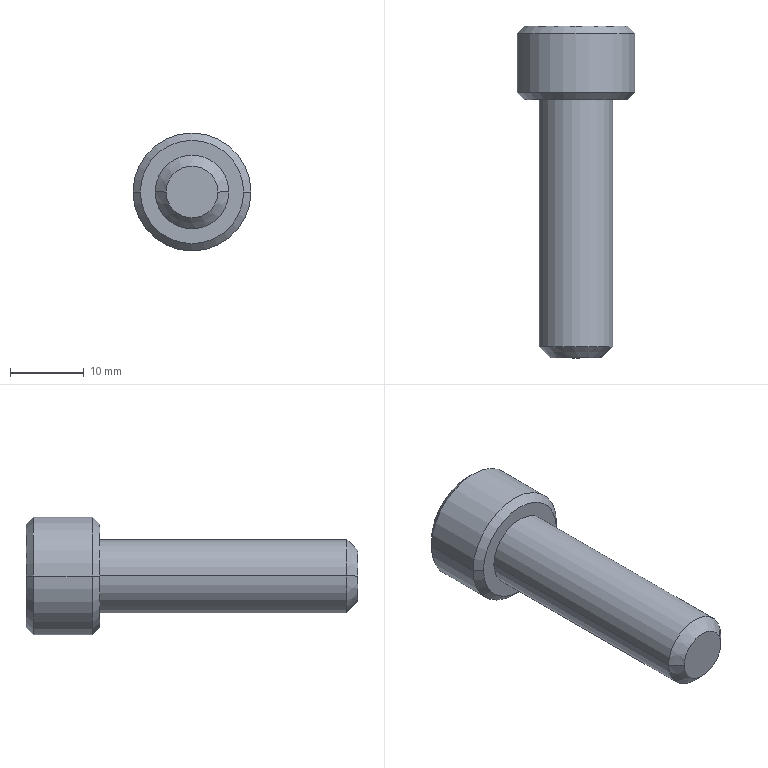Part | STEP file | BB62-M10-35L-1 | 1 solid | 27 faces | box 16 x 45 x 16 mm | volume 4350 mm3 | plane 15 | cone 8 | cylinder 4 | commonest cylinder face diameters 10 x2 16 x2
STEP:
#1=CARTESIAN_POINT('',(0.,2.359,0.));
#2=VERTEX_POINT('',#1);
#3=CARTESIAN_POINT('',(4.575,5.,0.));
#4=VERTEX_POINT('',#3);
#5=CARTESIAN_POINT('',(0.,2.359,0.));
#6=DIRECTION('',(0.866,0.5,0.));
#7=VECTOR('',#6,1000.);
#8=LINE('',#5,#7);
#9=EDGE_CURVE('',#2,#4,#8,.T.);
#10=ORIENTED_EDGE('',*,*,#9,.F.);
#11=CARTESIAN_POINT('',(-4.575,5.,0.));
#12=VERTEX_POINT('',#11);
#13=CARTESIAN_POINT('',(0.,2.359,0.));
#14=DIRECTION('',(-0.866,0.5,0.));
#15=VECTOR('',#14,1000.);
#16=LINE('',#13,#15);
#17=EDGE_CURVE('',#2,#12,#16,.T.);
#18=ORIENTED_EDGE('',*,*,#17,.T.);
#19=CARTESIAN_POINT('',(-3.962,5.,2.287));
#20=VERTEX_POINT('',#19);
#21=CARTESIAN_POINT('',(0.,5.,0.));
#22=DIRECTION('',(0.,-1.,0.));
#23=DIRECTION('',(-1.,0.,0.));
#24=AXIS2_PLACEMENT_3D('',#21,#22,#23);
#25=CIRCLE('',#24,4.575);
#26=EDGE_CURVE('',#20,#12,#25,.T.);
#27=ORIENTED_EDGE('',*,*,#26,.F.);
#28=CARTESIAN_POINT('',(0.,5.,4.575));
#29=VERTEX_POINT('',#28);
#30=CARTESIAN_POINT('',(0.,5.,0.));
#31=DIRECTION('',(0.,-1.,0.));
#32=DIRECTION('',(-1.,0.,0.));
#33=AXIS2_PLACEMENT_3D('',#30,#31,#32);
#34=CIRCLE('',#33,4.575);
#35=EDGE_CURVE('',#29,#20,#34,.T.);
#36=ORIENTED_EDGE('',*,*,#35,.F.);
#37=CARTESIAN_POINT('',(3.962,5.,2.287));
#38=VERTEX_POINT('',#37);
#39=CARTESIAN_POINT('',(0.,5.,0.));
#40=DIRECTION('',(0.,-1.,0.));
#41=DIRECTION('',(-1.,0.,0.));
#42=AXIS2_PLACEMENT_3D('',#39,#40,#41);
#43=CIRCLE('',#42,4.575);
#44=EDGE_CURVE('',#38,#29,#43,.T.);
#45=ORIENTED_EDGE('',*,*,#44,.F.);
#46=CARTESIAN_POINT('',(0.,5.,0.));
#47=DIRECTION('',(0.,-1.,0.));
#48=DIRECTION('',(-1.,0.,0.));
#49=AXIS2_PLACEMENT_3D('',#46,#47,#48);
#50=CIRCLE('',#49,4.575);
#51=EDGE_CURVE('',#4,#38,#50,.T.);
#52=ORIENTED_EDGE('',*,*,#51,.F.);
#53=EDGE_LOOP('',(#10,#18,#27,#36,#45,#52));
#54=FACE_OUTER_BOUND('',#53,.T.);
#55=CARTESIAN_POINT('',(0.,1002.359,0.));
#56=DIRECTION('',(0.,1.,0.));
#57=DIRECTION('',(1.,0.,0.));
#58=AXIS2_PLACEMENT_3D('',#55,#56,#57);
#59=CONICAL_SURFACE('',#58,1732.051,1.047);
#60=ADVANCED_FACE('',(#54),#59,.F.);
#61=CARTESIAN_POINT('',(3.5,-35.,0.));
#62=VERTEX_POINT('',#61);
#63=CARTESIAN_POINT('',(-3.5,-35.,0.));
#64=VERTEX_POINT('',#63);
#65=CARTESIAN_POINT('',(0.,-35.,0.));
#66=DIRECTION('',(0.,1.,0.));
#67=DIRECTION('',(1.,0.,0.));
#68=AXIS2_PLACEMENT_3D('',#65,#66,#67);
#69=CIRCLE('',#68,3.5);
#70=EDGE_CURVE('',#62,#64,#69,.T.);
#71=ORIENTED_EDGE('',*,*,#70,.T.);
#72=CARTESIAN_POINT('',(-5.,-33.5,0.));
#73=VERTEX_POINT('',#72);
#74=CARTESIAN_POINT('',(-3.5,-35.,0.));
#75=DIRECTION('',(-0.7071,0.7071,0.));
#76=VECTOR('',#75,1000.);
#77=LINE('',#74,#76);
#78=EDGE_CURVE('',#64,#73,#77,.T.);
#79=ORIENTED_EDGE('',*,*,#78,.T.);
#80=CARTESIAN_POINT('',(5.,-33.5,0.));
#81=VERTEX_POINT('',#80);
#82=CARTESIAN_POINT('',(0.,-33.5,0.));
#83=DIRECTION('',(0.,-1.,0.));
#84=DIRECTION('',(-1.,0.,0.));
#85=AXIS2_PLACEMENT_3D('',#82,#83,#84);
#86=CIRCLE('',#85,5.);
#87=EDGE_CURVE('',#73,#81,#86,.T.);
#88=ORIENTED_EDGE('',*,*,#87,.T.);
#89=CARTESIAN_POINT('',(3.5,-35.,0.));
#90=DIRECTION('',(0.7071,0.7071,0.));
#91=VECTOR('',#90,1000.);
#92=LINE('',#89,#91);
#93=EDGE_CURVE('',#62,#81,#92,.T.);
#94=ORIENTED_EDGE('',*,*,#93,.F.);
#95=EDGE_LOOP('',(#71,#79,#88,#94));
#96=FACE_OUTER_BOUND('',#95,.T.);
#97=CARTESIAN_POINT('',(0.,-35.,0.));
#98=DIRECTION('',(0.,1.,0.));
#99=DIRECTION('',(1.,0.,0.));
#100=AXIS2_PLACEMENT_3D('',#97,#98,#99);
#101=CONICAL_SURFACE('',#100,3.5,0.7854);
#102=ADVANCED_FACE('',(#96),#101,.T.);
#103=ORIENTED_EDGE('',*,*,#87,.F.);
#104=CARTESIAN_POINT('',(-5.,0.,0.));
#105=VERTEX_POINT('',#104);
#106=CARTESIAN_POINT('',(-5.,-33.5,0.));
#107=DIRECTION('',(0.,1.,0.));
#108=VECTOR('',#107,1000.);
#109=LINE('',#106,#108);
#110=EDGE_CURVE('',#73,#105,#109,.T.);
#111=ORIENTED_EDGE('',*,*,#110,.T.);
#112=CARTESIAN_POINT('',(5.,0.,0.));
#113=VERTEX_POINT('',#112);
#114=CARTESIAN_POINT('',(0.,0.,0.));
#115=DIRECTION('',(0.,-1.,0.));
#116=DIRECTION('',(-1.,0.,0.));
#117=AXIS2_PLACEMENT_3D('',#114,#115,#116);
#118=CIRCLE('',#117,5.);
#119=EDGE_CURVE('',#105,#113,#118,.T.);
#120=ORIENTED_EDGE('',*,*,#119,.T.);
#121=CARTESIAN_POINT('',(5.,-33.5,0.));
#122=DIRECTION('',(0.,1.,0.));
#123=VECTOR('',#122,1000.);
#124=LINE('',#121,#123);
#125=EDGE_CURVE('',#81,#113,#124,.T.);
#126=ORIENTED_EDGE('',*,*,#125,.F.);
#127=EDGE_LOOP('',(#103,#111,#120,#126));
#128=FACE_OUTER_BOUND('',#127,.T.);
#129=CARTESIAN_POINT('',(0.,-33.5,0.));
#130=DIRECTION('',(0.,1.,0.));
#131=DIRECTION('',(1.,0.,0.));
#132=AXIS2_PLACEMENT_3D('',#129,#130,#131);
#133=CYLINDRICAL_SURFACE('',#132,5.);
#134=ADVANCED_FACE('',(#128),#133,.T.);
#135=CARTESIAN_POINT('',(-7.,10.,0.));
#136=VERTEX_POINT('',#135);
#137=CARTESIAN_POINT('',(7.,10.,0.));
#138=VERTEX_POINT('',#137);
#139=CARTESIAN_POINT('',(0.,10.,0.));
#140=DIRECTION('',(0.,-1.,0.));
#141=DIRECTION('',(-1.,0.,0.));
#142=AXIS2_PLACEMENT_3D('',#139,#140,#141);
#143=CIRCLE('',#142,7.);
#144=EDGE_CURVE('',#136,#138,#143,.T.);
#145=ORIENTED_EDGE('',*,*,#144,.T.);
#146=CARTESIAN_POINT('',(8.,9.,0.));
#147=VERTEX_POINT('',#146);
#148=CARTESIAN_POINT('',(8.,9.,0.));
#149=DIRECTION('',(0.7071,-0.7071,0.));
#150=VECTOR('',#149,1000.);
#151=LINE('',#148,#150);
#152=EDGE_CURVE('',#138,#147,#151,.T.);
#153=ORIENTED_EDGE('',*,*,#152,.T.);
#154=CARTESIAN_POINT('',(-8.,9.,0.));
#155=VERTEX_POINT('',#154);
#156=CARTESIAN_POINT('',(0.,9.,0.));
#157=DIRECTION('',(0.,-1.,0.));
#158=DIRECTION('',(-1.,0.,0.));
#159=AXIS2_PLACEMENT_3D('',#156,#157,#158);
#160=CIRCLE('',#159,8.);
#161=EDGE_CURVE('',#155,#147,#160,.T.);
#162=ORIENTED_EDGE('',*,*,#161,.F.);
#163=CARTESIAN_POINT('',(-8.,9.,0.));
#164=DIRECTION('',(-0.7071,-0.7071,0.));
#165=VECTOR('',#164,1000.);
#166=LINE('',#163,#165);
#167=EDGE_CURVE('',#136,#155,#166,.T.);
#168=ORIENTED_EDGE('',*,*,#167,.F.);
#169=EDGE_LOOP('',(#145,#153,#162,#168));
#170=FACE_OUTER_BOUND('',#169,.T.);
#171=CARTESIAN_POINT('',(0.,9.,0.));
#172=DIRECTION('',(0.,-1.,0.));
#173=DIRECTION('',(-1.,0.,0.));
#174=AXIS2_PLACEMENT_3D('',#171,#172,#173);
#175=CONICAL_SURFACE('',#174,8.,0.7854);
#176=ADVANCED_FACE('',(#170),#175,.T.);
#177=ORIENTED_EDGE('',*,*,#161,.T.);
#178=CARTESIAN_POINT('',(8.,1.,0.));
#179=VERTEX_POINT('',#178);
#180=CARTESIAN_POINT('',(8.,1.62,0.));
#181=DIRECTION('',(0.,-1.,0.));
#182=VECTOR('',#181,1000.);
#183=LINE('',#180,#182);
#184=EDGE_CURVE('',#147,#179,#183,.T.);
#185=ORIENTED_EDGE('',*,*,#184,.T.);
#186=CARTESIAN_POINT('',(-8.,1.,0.));
#187=VERTEX_POINT('',#186);
#188=CARTESIAN_POINT('',(0.,1.,0.));
#189=DIRECTION('',(0.,-1.,0.));
#190=DIRECTION('',(-1.,0.,0.));
#191=AXIS2_PLACEMENT_3D('',#188,#189,#190);
#192=CIRCLE('',#191,8.);
#193=EDGE_CURVE('',#187,#179,#192,.T.);
#194=ORIENTED_EDGE('',*,*,#193,.F.);
#195=CARTESIAN_POINT('',(-8.,1.62,0.));
#196=DIRECTION('',(0.,-1.,0.));
#197=VECTOR('',#196,1000.);
#198=LINE('',#195,#197);
#199=EDGE_CURVE('',#155,#187,#198,.T.);
#200=ORIENTED_EDGE('',*,*,#199,.F.);
#201=EDGE_LOOP('',(#177,#185,#194,#200));
#202=FACE_OUTER_BOUND('',#201,.T.);
#203=CARTESIAN_POINT('',(0.,1.62,0.));
#204=DIRECTION('',(0.,-1.,0.));
#205=DIRECTION('',(-1.,0.,0.));
#206=AXIS2_PLACEMENT_3D('',#203,#204,#205);
#207=CYLINDRICAL_SURFACE('',#206,8.);
#208=ADVANCED_FACE('',(#202),#207,.T.);
#209=CARTESIAN_POINT('',(-7.,0.,0.));
#210=VERTEX_POINT('',#209);
#211=CARTESIAN_POINT('',(7.,0.,0.));
#212=VERTEX_POINT('',#211);
#213=CARTESIAN_POINT('',(0.,0.,0.));
#214=DIRECTION('',(0.,-1.,0.));
#215=DIRECTION('',(-1.,0.,0.));
#216=AXIS2_PLACEMENT_3D('',#213,#214,#215);
#217=CIRCLE('',#216,7.);
#218=EDGE_CURVE('',#210,#212,#217,.T.);
#219=ORIENTED_EDGE('',*,*,#218,.F.);
#220=CARTESIAN_POINT('',(-7.,0.,0.));
#221=DIRECTION('',(-0.7071,0.7071,0.));
#222=VECTOR('',#221,1000.);
#223=LINE('',#220,#222);
#224=EDGE_CURVE('',#210,#187,#223,.T.);
#225=ORIENTED_EDGE('',*,*,#224,.T.);
#226=ORIENTED_EDGE('',*,*,#193,.T.);
#227=CARTESIAN_POINT('',(7.,0.,0.));
#228=DIRECTION('',(0.7071,0.7071,0.));
#229=VECTOR('',#228,1000.);
#230=LINE('',#227,#229);
#231=EDGE_CURVE('',#212,#179,#230,.T.);
#232=ORIENTED_EDGE('',*,*,#231,.F.);
#233=EDGE_LOOP('',(#219,#225,#226,#232));
#234=FACE_OUTER_BOUND('',#233,.T.);
#235=CARTESIAN_POINT('',(0.,0.,0.));
#236=DIRECTION('',(0.,1.,0.));
#237=DIRECTION('',(1.,0.,0.));
#238=AXIS2_PLACEMENT_3D('',#235,#236,#237);
#239=CONICAL_SURFACE('',#238,7.,0.7854);
#240=ADVANCED_FACE('',(#234),#239,.T.);
#241=ORIENTED_EDGE('',*,*,#144,.F.);
#242=CARTESIAN_POINT('',(0.,10.,0.));
#243=DIRECTION('',(0.,-1.,0.));
#244=DIRECTION('',(-1.,0.,0.));
#245=AXIS2_PLACEMENT_3D('',#242,#243,#244);
#246=CIRCLE('',#245,7.);
#247=EDGE_CURVE('',#138,#136,#246,.T.);
#248=ORIENTED_EDGE('',*,*,#247,.F.);
#249=EDGE_LOOP('',(#241,#248));
#250=FACE_OUTER_BOUND('',#249,.T.);
#251=CARTESIAN_POINT('',(0.,10.,-4.575));
#252=VERTEX_POINT('',#251);
#253=CARTESIAN_POINT('',(-3.962,10.,-2.288));
#254=VERTEX_POINT('',#253);
#255=CARTESIAN_POINT('',(0.,10.,-4.575));
#256=DIRECTION('',(-0.866,0.,0.5));
#257=VECTOR('',#256,1000.);
#258=LINE('',#255,#257);
#259=EDGE_CURVE('',#252,#254,#258,.T.);
#260=ORIENTED_EDGE('',*,*,#259,.F.);
#261=CARTESIAN_POINT('',(3.962,10.,-2.288));
#262=VERTEX_POINT('',#261);
#263=CARTESIAN_POINT('',(3.962,10.,-2.288));
#264=DIRECTION('',(-0.866,0.,-0.5));
#265=VECTOR('',#264,1000.);
#266=LINE('',#263,#265);
#267=EDGE_CURVE('',#262,#252,#266,.T.);
#268=ORIENTED_EDGE('',*,*,#267,.F.);
#269=CARTESIAN_POINT('',(3.962,10.,2.287));
#270=VERTEX_POINT('',#269);
#271=CARTESIAN_POINT('',(3.962,10.,2.287));
#272=DIRECTION('',(0.,0.,-1.));
#273=VECTOR('',#272,1000.);
#274=LINE('',#271,#273);
#275=EDGE_CURVE('',#270,#262,#274,.T.);
#276=ORIENTED_EDGE('',*,*,#275,.F.);
#277=CARTESIAN_POINT('',(0.,10.,4.575));
#278=VERTEX_POINT('',#277);
#279=CARTESIAN_POINT('',(0.,10.,4.575));
#280=DIRECTION('',(0.866,0.,-0.5));
#281=VECTOR('',#280,1000.);
#282=LINE('',#279,#281);
#283=EDGE_CURVE('',#278,#270,#282,.T.);
#284=ORIENTED_EDGE('',*,*,#283,.F.);
#285=CARTESIAN_POINT('',(-3.962,10.,2.287));
#286=VERTEX_POINT('',#285);
#287=CARTESIAN_POINT('',(-3.962,10.,2.287));
#288=DIRECTION('',(0.866,0.,0.5));
#289=VECTOR('',#288,1000.);
#290=LINE('',#287,#289);
#291=EDGE_CURVE('',#286,#278,#290,.T.);
#292=ORIENTED_EDGE('',*,*,#291,.F.);
#293=CARTESIAN_POINT('',(-3.962,10.,-2.288));
#294=DIRECTION('',(0.,0.,1.));
#295=VECTOR('',#294,1000.);
#296=LINE('',#293,#295);
#297=EDGE_CURVE('',#254,#286,#296,.T.);
#298=ORIENTED_EDGE('',*,*,#297,.F.);
#299=EDGE_LOOP('',(#260,#268,#276,#284,#292,#298));
#300=FACE_BOUND('',#299,.T.);
#301=CARTESIAN_POINT('',(7.,10.,0.));
#302=DIRECTION('',(0.,1.,0.));
#303=DIRECTION('',(1.,0.,0.));
#304=AXIS2_PLACEMENT_3D('',#301,#302,#303);
#305=PLANE('',#304);
#306=ADVANCED_FACE('',(#250,#300),#305,.T.);
#307=CARTESIAN_POINT('',(0.,0.,0.));
#308=DIRECTION('',(0.,-1.,0.));
#309=DIRECTION('',(-1.,0.,0.));
#310=AXIS2_PLACEMENT_3D('',#307,#308,#309);
#311=CIRCLE('',#310,5.);
#312=EDGE_CURVE('',#113,#105,#311,.T.);
#313=ORIENTED_EDGE('',*,*,#312,.F.);
#314=ORIENTED_EDGE('',*,*,#119,.F.);
#315=EDGE_LOOP('',(#313,#314));
#316=FACE_BOUND('',#315,.T.);
#317=CARTESIAN_POINT('',(0.,0.,0.));
#318=DIRECTION('',(0.,-1.,0.));
#319=DIRECTION('',(-1.,0.,0.));
#320=AXIS2_PLACEMENT_3D('',#317,#318,#319);
#321=CIRCLE('',#320,7.);
#322=EDGE_CURVE('',#212,#210,#321,.T.);
#323=ORIENTED_EDGE('',*,*,#322,.T.);
#324=ORIENTED_EDGE('',*,*,#218,.T.);
#325=EDGE_LOOP('',(#323,#324));
#326=FACE_OUTER_BOUND('',#325,.T.);
#327=CARTESIAN_POINT('',(0.,0.,0.));
#328=DIRECTION('',(0.,-1.,0.));
#329=DIRECTION('',(-1.,0.,0.));
#330=AXIS2_PLACEMENT_3D('',#327,#328,#329);
#331=PLANE('',#330);
#332=ADVANCED_FACE('',(#316,#326),#331,.T.);
#333=ORIENTED_EDGE('',*,*,#224,.F.);
#334=ORIENTED_EDGE('',*,*,#322,.F.);
#335=ORIENTED_EDGE('',*,*,#231,.T.);
#336=CARTESIAN_POINT('',(0.,1.,0.));
#337=DIRECTION('',(0.,-1.,0.));
#338=DIRECTION('',(-1.,0.,0.));
#339=AXIS2_PLACEMENT_3D('',#336,#337,#338);
#340=CIRCLE('',#339,8.);
#341=EDGE_CURVE('',#179,#187,#340,.T.);
#342=ORIENTED_EDGE('',*,*,#341,.T.);
#343=EDGE_LOOP('',(#333,#334,#335,#342));
#344=FACE_OUTER_BOUND('',#343,.T.);
#345=CARTESIAN_POINT('',(0.,0.,0.));
#346=DIRECTION('',(0.,1.,0.));
#347=DIRECTION('',(1.,0.,0.));
#348=AXIS2_PLACEMENT_3D('',#345,#346,#347);
#349=CONICAL_SURFACE('',#348,7.,0.7854);
#350=ADVANCED_FACE('',(#344),#349,.T.);
#351=ORIENTED_EDGE('',*,*,#184,.F.);
#352=CARTESIAN_POINT('',(0.,9.,0.));
#353=DIRECTION('',(0.,-1.,0.));
#354=DIRECTION('',(-1.,0.,0.));
#355=AXIS2_PLACEMENT_3D('',#352,#353,#354);
#356=CIRCLE('',#355,8.);
#357=EDGE_CURVE('',#147,#155,#356,.T.);
#358=ORIENTED_EDGE('',*,*,#357,.T.);
#359=ORIENTED_EDGE('',*,*,#199,.T.);
#360=ORIENTED_EDGE('',*,*,#341,.F.);
#361=EDGE_LOOP('',(#351,#358,#359,#360));
#362=FACE_OUTER_BOUND('',#361,.T.);
#363=CARTESIAN_POINT('',(0.,1.62,0.));
#364=DIRECTION('',(0.,-1.,0.));
#365=DIRECTION('',(-1.,0.,0.));
#366=AXIS2_PLACEMENT_3D('',#363,#364,#365);
#367=CYLINDRICAL_SURFACE('',#366,8.);
#368=ADVANCED_FACE('',(#362),#367,.T.);
#369=ORIENTED_EDGE('',*,*,#152,.F.);
#370=ORIENTED_EDGE('',*,*,#247,.T.);
#371=ORIENTED_EDGE('',*,*,#167,.T.);
#372=ORIENTED_EDGE('',*,*,#357,.F.);
#373=EDGE_LOOP('',(#369,#370,#371,#372));
#374=FACE_OUTER_BOUND('',#373,.T.);
#375=CARTESIAN_POINT('',(0.,9.,0.));
#376=DIRECTION('',(0.,-1.,0.));
#377=DIRECTION('',(-1.,0.,0.));
#378=AXIS2_PLACEMENT_3D('',#375,#376,#377);
#379=CONICAL_SURFACE('',#378,8.,0.7854);
#380=ADVANCED_FACE('',(#374),#379,.T.);
#381=ORIENTED_EDGE('',*,*,#110,.F.);
#382=CARTESIAN_POINT('',(0.,-33.5,0.));
#383=DIRECTION('',(0.,-1.,0.));
#384=DIRECTION('',(-1.,0.,0.));
#385=AXIS2_PLACEMENT_3D('',#382,#383,#384);
#386=CIRCLE('',#385,5.);
#387=EDGE_CURVE('',#81,#73,#386,.T.);
#388=ORIENTED_EDGE('',*,*,#387,.F.);
#389=ORIENTED_EDGE('',*,*,#125,.T.);
#390=ORIENTED_EDGE('',*,*,#312,.T.);
#391=EDGE_LOOP('',(#381,#388,#389,#390));
#392=FACE_OUTER_BOUND('',#391,.T.);
#393=CARTESIAN_POINT('',(0.,-33.5,0.));
#394=DIRECTION('',(0.,1.,0.));
#395=DIRECTION('',(1.,0.,0.));
#396=AXIS2_PLACEMENT_3D('',#393,#394,#395);
#397=CYLINDRICAL_SURFACE('',#396,5.);
#398=ADVANCED_FACE('',(#392),#397,.T.);
#399=ORIENTED_EDGE('',*,*,#70,.F.);
#400=CARTESIAN_POINT('',(0.,-35.,0.));
#401=DIRECTION('',(0.,1.,0.));
#402=DIRECTION('',(1.,0.,0.));
#403=AXIS2_PLACEMENT_3D('',#400,#401,#402);
#404=CIRCLE('',#403,3.5);
#405=EDGE_CURVE('',#64,#62,#404,.T.);
#406=ORIENTED_EDGE('',*,*,#405,.F.);
#407=EDGE_LOOP('',(#399,#406));
#408=FACE_OUTER_BOUND('',#407,.T.);
#409=CARTESIAN_POINT('',(0.,-35.,0.));
#410=DIRECTION('',(0.,-1.,0.));
#411=DIRECTION('',(-1.,0.,0.));
#412=AXIS2_PLACEMENT_3D('',#409,#410,#411);
#413=PLANE('',#412);
#414=ADVANCED_FACE('',(#408),#413,.T.);
#415=ORIENTED_EDGE('',*,*,#78,.F.);
#416=ORIENTED_EDGE('',*,*,#405,.T.);
#417=ORIENTED_EDGE('',*,*,#93,.T.);
#418=ORIENTED_EDGE('',*,*,#387,.T.);
#419=EDGE_LOOP('',(#415,#416,#417,#418));
#420=FACE_OUTER_BOUND('',#419,.T.);
#421=CARTESIAN_POINT('',(0.,-35.,0.));
#422=DIRECTION('',(0.,1.,0.));
#423=DIRECTION('',(1.,0.,0.));
#424=AXIS2_PLACEMENT_3D('',#421,#422,#423);
#425=CONICAL_SURFACE('',#424,3.5,0.7854);
#426=ADVANCED_FACE('',(#420),#425,.T.);
#427=CARTESIAN_POINT('',(3.962,5.,-2.288));
#428=VERTEX_POINT('',#427);
#429=CARTESIAN_POINT('',(0.,5.,-4.575));
#430=VERTEX_POINT('',#429);
#431=CARTESIAN_POINT('',(3.962,5.,-2.288));
#432=DIRECTION('',(-0.866,0.,-0.5));
#433=VECTOR('',#432,1000.);
#434=LINE('',#431,#433);
#435=EDGE_CURVE('',#428,#430,#434,.T.);
#436=ORIENTED_EDGE('',*,*,#435,.F.);
#437=CARTESIAN_POINT('',(3.962,10.,-2.288));
#438=DIRECTION('',(0.,-1.,0.));
#439=VECTOR('',#438,1000.);
#440=LINE('',#437,#439);
#441=EDGE_CURVE('',#262,#428,#440,.T.);
#442=ORIENTED_EDGE('',*,*,#441,.F.);
#443=ORIENTED_EDGE('',*,*,#267,.T.);
#444=CARTESIAN_POINT('',(0.,10.,-4.575));
#445=DIRECTION('',(0.,-1.,0.));
#446=VECTOR('',#445,1000.);
#447=LINE('',#444,#446);
#448=EDGE_CURVE('',#252,#430,#447,.T.);
#449=ORIENTED_EDGE('',*,*,#448,.T.);
#450=EDGE_LOOP('',(#436,#442,#443,#449));
#451=FACE_OUTER_BOUND('',#450,.T.);
#452=CARTESIAN_POINT('',(3.962,10.,-2.288));
#453=DIRECTION('',(-0.5,0.,0.866));
#454=DIRECTION('',(0.866,0.,0.5));
#455=AXIS2_PLACEMENT_3D('',#452,#453,#454);
#456=PLANE('',#455);
#457=ADVANCED_FACE('',(#451),#456,.T.);
#458=CARTESIAN_POINT('',(-3.962,5.,-2.288));
#459=VERTEX_POINT('',#458);
#460=CARTESIAN_POINT('',(0.,5.,-4.575));
#461=DIRECTION('',(-0.866,0.,0.5));
#462=VECTOR('',#461,1000.);
#463=LINE('',#460,#462);
#464=EDGE_CURVE('',#430,#459,#463,.T.);
#465=ORIENTED_EDGE('',*,*,#464,.F.);
#466=ORIENTED_EDGE('',*,*,#448,.F.);
#467=ORIENTED_EDGE('',*,*,#259,.T.);
#468=CARTESIAN_POINT('',(-3.962,10.,-2.288));
#469=DIRECTION('',(0.,-1.,0.));
#470=VECTOR('',#469,1000.);
#471=LINE('',#468,#470);
#472=EDGE_CURVE('',#254,#459,#471,.T.);
#473=ORIENTED_EDGE('',*,*,#472,.T.);
#474=EDGE_LOOP('',(#465,#466,#467,#473));
#475=FACE_OUTER_BOUND('',#474,.T.);
#476=CARTESIAN_POINT('',(0.,10.,-4.575));
#477=DIRECTION('',(0.5,0.,0.866));
#478=DIRECTION('',(0.866,0.,-0.5));
#479=AXIS2_PLACEMENT_3D('',#476,#477,#478);
#480=PLANE('',#479);
#481=ADVANCED_FACE('',(#475),#480,.T.);
#482=CARTESIAN_POINT('',(-3.962,5.,-2.288));
#483=DIRECTION('',(0.,0.,1.));
#484=VECTOR('',#483,1000.);
#485=LINE('',#482,#484);
#486=EDGE_CURVE('',#459,#20,#485,.T.);
#487=ORIENTED_EDGE('',*,*,#486,.F.);
#488=ORIENTED_EDGE('',*,*,#472,.F.);
#489=ORIENTED_EDGE('',*,*,#297,.T.);
#490=CARTESIAN_POINT('',(-3.962,10.,2.287));
#491=DIRECTION('',(0.,-1.,0.));
#492=VECTOR('',#491,1000.);
#493=LINE('',#490,#492);
#494=EDGE_CURVE('',#286,#20,#493,.T.);
#495=ORIENTED_EDGE('',*,*,#494,.T.);
#496=EDGE_LOOP('',(#487,#488,#489,#495));
#497=FACE_OUTER_BOUND('',#496,.T.);
#498=CARTESIAN_POINT('',(-3.962,10.,-2.288));
#499=DIRECTION('',(1.,0.,0.));
#500=DIRECTION('',(0.,0.,-1.));
#501=AXIS2_PLACEMENT_3D('',#498,#499,#500);
#502=PLANE('',#501);
#503=ADVANCED_FACE('',(#497),#502,.T.);
#504=CARTESIAN_POINT('',(-3.962,5.,2.287));
#505=DIRECTION('',(0.866,0.,0.5));
#506=VECTOR('',#505,1000.);
#507=LINE('',#504,#506);
#508=EDGE_CURVE('',#20,#29,#507,.T.);
#509=ORIENTED_EDGE('',*,*,#508,.F.);
#510=ORIENTED_EDGE('',*,*,#494,.F.);
#511=ORIENTED_EDGE('',*,*,#291,.T.);
#512=CARTESIAN_POINT('',(0.,10.,4.575));
#513=DIRECTION('',(0.,-1.,0.));
#514=VECTOR('',#513,1000.);
#515=LINE('',#512,#514);
#516=EDGE_CURVE('',#278,#29,#515,.T.);
#517=ORIENTED_EDGE('',*,*,#516,.T.);
#518=EDGE_LOOP('',(#509,#510,#511,#517));
#519=FACE_OUTER_BOUND('',#518,.T.);
#520=CARTESIAN_POINT('',(-3.962,10.,2.287));
#521=DIRECTION('',(0.5,0.,-0.866));
#522=DIRECTION('',(-0.866,0.,-0.5));
#523=AXIS2_PLACEMENT_3D('',#520,#521,#522);
#524=PLANE('',#523);
#525=ADVANCED_FACE('',(#519),#524,.T.);
#526=CARTESIAN_POINT('',(0.,5.,4.575));
#527=DIRECTION('',(0.866,0.,-0.5));
#528=VECTOR('',#527,1000.);
#529=LINE('',#526,#528);
#530=EDGE_CURVE('',#29,#38,#529,.T.);
#531=ORIENTED_EDGE('',*,*,#530,.F.);
#532=ORIENTED_EDGE('',*,*,#516,.F.);
#533=ORIENTED_EDGE('',*,*,#283,.T.);
#534=CARTESIAN_POINT('',(3.962,10.,2.287));
#535=DIRECTION('',(0.,-1.,0.));
#536=VECTOR('',#535,1000.);
#537=LINE('',#534,#536);
#538=EDGE_CURVE('',#270,#38,#537,.T.);
#539=ORIENTED_EDGE('',*,*,#538,.T.);
#540=EDGE_LOOP('',(#531,#532,#533,#539));
#541=FACE_OUTER_BOUND('',#540,.T.);
#542=CARTESIAN_POINT('',(0.,10.,4.575));
#543=DIRECTION('',(-0.5,0.,-0.866));
#544=DIRECTION('',(-0.866,0.,0.5));
#545=AXIS2_PLACEMENT_3D('',#542,#543,#544);
#546=PLANE('',#545);
#547=ADVANCED_FACE('',(#541),#546,.T.);
#548=CARTESIAN_POINT('',(3.962,5.,2.287));
#549=DIRECTION('',(0.,0.,-1.));
#550=VECTOR('',#549,1000.);
#551=LINE('',#548,#550);
#552=EDGE_CURVE('',#38,#428,#551,.T.);
#553=ORIENTED_EDGE('',*,*,#552,.F.);
#554=ORIENTED_EDGE('',*,*,#538,.F.);
#555=ORIENTED_EDGE('',*,*,#275,.T.);
#556=ORIENTED_EDGE('',*,*,#441,.T.);
#557=EDGE_LOOP('',(#553,#554,#555,#556));
#558=FACE_OUTER_BOUND('',#557,.T.);
#559=CARTESIAN_POINT('',(3.962,10.,2.287));
#560=DIRECTION('',(-1.,0.,0.));
#561=DIRECTION('',(0.,0.,1.));
#562=AXIS2_PLACEMENT_3D('',#559,#560,#561);
#563=PLANE('',#562);
#564=ADVANCED_FACE('',(#558),#563,.T.);
#565=ORIENTED_EDGE('',*,*,#435,.T.);
#566=CARTESIAN_POINT('',(0.,5.,0.));
#567=DIRECTION('',(0.,-1.,0.));
#568=DIRECTION('',(-1.,0.,0.));
#569=AXIS2_PLACEMENT_3D('',#566,#567,#568);
#570=CIRCLE('',#569,4.575);
#571=EDGE_CURVE('',#430,#428,#570,.T.);
#572=ORIENTED_EDGE('',*,*,#571,.T.);
#573=EDGE_LOOP('',(#565,#572));
#574=FACE_OUTER_BOUND('',#573,.T.);
#575=CARTESIAN_POINT('',(0.,5.,0.));
#576=DIRECTION('',(0.,1.,0.));
#577=DIRECTION('',(1.,0.,0.));
#578=AXIS2_PLACEMENT_3D('',#575,#576,#577);
#579=PLANE('',#578);
#580=ADVANCED_FACE('',(#574),#579,.F.);
#581=ORIENTED_EDGE('',*,*,#552,.T.);
#582=CARTESIAN_POINT('',(0.,5.,0.));
#583=DIRECTION('',(0.,-1.,0.));
#584=DIRECTION('',(-1.,0.,0.));
#585=AXIS2_PLACEMENT_3D('',#582,#583,#584);
#586=CIRCLE('',#585,4.575);
#587=EDGE_CURVE('',#428,#4,#586,.T.);
#588=ORIENTED_EDGE('',*,*,#587,.T.);
#589=ORIENTED_EDGE('',*,*,#51,.T.);
#590=EDGE_LOOP('',(#581,#588,#589));
#591=FACE_OUTER_BOUND('',#590,.T.);
#592=CARTESIAN_POINT('',(0.,5.,0.));
#593=DIRECTION('',(0.,1.,0.));
#594=DIRECTION('',(1.,0.,0.));
#595=AXIS2_PLACEMENT_3D('',#592,#593,#594);
#596=PLANE('',#595);
#597=ADVANCED_FACE('',(#591),#596,.F.);
#598=ORIENTED_EDGE('',*,*,#530,.T.);
#599=ORIENTED_EDGE('',*,*,#44,.T.);
#600=EDGE_LOOP('',(#598,#599));
#601=FACE_OUTER_BOUND('',#600,.T.);
#602=CARTESIAN_POINT('',(0.,5.,0.));
#603=DIRECTION('',(0.,1.,0.));
#604=DIRECTION('',(1.,0.,0.));
#605=AXIS2_PLACEMENT_3D('',#602,#603,#604);
#606=PLANE('',#605);
#607=ADVANCED_FACE('',(#601),#606,.F.);
#608=ORIENTED_EDGE('',*,*,#508,.T.);
#609=ORIENTED_EDGE('',*,*,#35,.T.);
#610=EDGE_LOOP('',(#608,#609));
#611=FACE_OUTER_BOUND('',#610,.T.);
#612=CARTESIAN_POINT('',(0.,5.,0.));
#613=DIRECTION('',(0.,1.,0.));
#614=DIRECTION('',(1.,0.,0.));
#615=AXIS2_PLACEMENT_3D('',#612,#613,#614);
#616=PLANE('',#615);
#617=ADVANCED_FACE('',(#611),#616,.F.);
#618=ORIENTED_EDGE('',*,*,#486,.T.);
#619=ORIENTED_EDGE('',*,*,#26,.T.);
#620=CARTESIAN_POINT('',(0.,5.,0.));
#621=DIRECTION('',(0.,-1.,0.));
#622=DIRECTION('',(-1.,0.,0.));
#623=AXIS2_PLACEMENT_3D('',#620,#621,#622);
#624=CIRCLE('',#623,4.575);
#625=EDGE_CURVE('',#12,#459,#624,.T.);
#626=ORIENTED_EDGE('',*,*,#625,.T.);
#627=EDGE_LOOP('',(#618,#619,#626));
#628=FACE_OUTER_BOUND('',#627,.T.);
#629=CARTESIAN_POINT('',(0.,5.,0.));
#630=DIRECTION('',(0.,1.,0.));
#631=DIRECTION('',(1.,0.,0.));
#632=AXIS2_PLACEMENT_3D('',#629,#630,#631);
#633=PLANE('',#632);
#634=ADVANCED_FACE('',(#628),#633,.F.);
#635=ORIENTED_EDGE('',*,*,#464,.T.);
#636=CARTESIAN_POINT('',(0.,5.,0.));
#637=DIRECTION('',(0.,-1.,0.));
#638=DIRECTION('',(-1.,0.,0.));
#639=AXIS2_PLACEMENT_3D('',#636,#637,#638);
#640=CIRCLE('',#639,4.575);
#641=EDGE_CURVE('',#459,#430,#640,.T.);
#642=ORIENTED_EDGE('',*,*,#641,.T.);
#643=EDGE_LOOP('',(#635,#642));
#644=FACE_OUTER_BOUND('',#643,.T.);
#645=CARTESIAN_POINT('',(0.,5.,0.));
#646=DIRECTION('',(0.,1.,0.));
#647=DIRECTION('',(1.,0.,0.));
#648=AXIS2_PLACEMENT_3D('',#645,#646,#647);
#649=PLANE('',#648);
#650=ADVANCED_FACE('',(#644),#649,.F.);
#651=ORIENTED_EDGE('',*,*,#17,.F.);
#652=ORIENTED_EDGE('',*,*,#9,.T.);
#653=ORIENTED_EDGE('',*,*,#587,.F.);
#654=ORIENTED_EDGE('',*,*,#571,.F.);
#655=ORIENTED_EDGE('',*,*,#641,.F.);
#656=ORIENTED_EDGE('',*,*,#625,.F.);
#657=EDGE_LOOP('',(#651,#652,#653,#654,#655,#656));
#658=FACE_OUTER_BOUND('',#657,.T.);
#659=CARTESIAN_POINT('',(0.,1002.359,0.));
#660=DIRECTION('',(0.,1.,0.));
#661=DIRECTION('',(1.,0.,0.));
#662=AXIS2_PLACEMENT_3D('',#659,#660,#661);
#663=CONICAL_SURFACE('',#662,1732.051,1.047);
#664=ADVANCED_FACE('',(#658),#663,.F.);
#665=CLOSED_SHELL('',(#60,#102,#134,#176,#208,#240,#306,#332,#350,#368,#380,#398,#414,#426,#457,#481,#503,#525,#547,#564,#580,#597,#607,#617,#634,#650,#664));
#666=MANIFOLD_SOLID_BREP('',#665);
#667=CARTESIAN_POINT('',(0.,0.,0.));
#668=DIRECTION('',(0.,0.,1.));
#669=DIRECTION('',(1.,0.,0.));
#670=AXIS2_PLACEMENT_3D('',#667,#668,#669);
#671=(LENGTH_UNIT()NAMED_UNIT(*)SI_UNIT(.MILLI.,.METRE.));
#672=UNCERTAINTY_MEASURE_WITH_UNIT(LENGTH_MEASURE(0.00001),#671,'','');
#673=(NAMED_UNIT(*)PLANE_ANGLE_UNIT()SI_UNIT($,.RADIAN.));
#674=(NAMED_UNIT(*)SI_UNIT($,.STERADIAN.)SOLID_ANGLE_UNIT());
#675=(GEOMETRIC_REPRESENTATION_CONTEXT(3)GLOBAL_UNCERTAINTY_ASSIGNED_CONTEXT((#672))GLOBAL_UNIT_ASSIGNED_CONTEXT((#671,#673,#674))REPRESENTATION_CONTEXT('',''));
#676=ADVANCED_BREP_SHAPE_REPRESENTATION('',(#666,#670),#675);